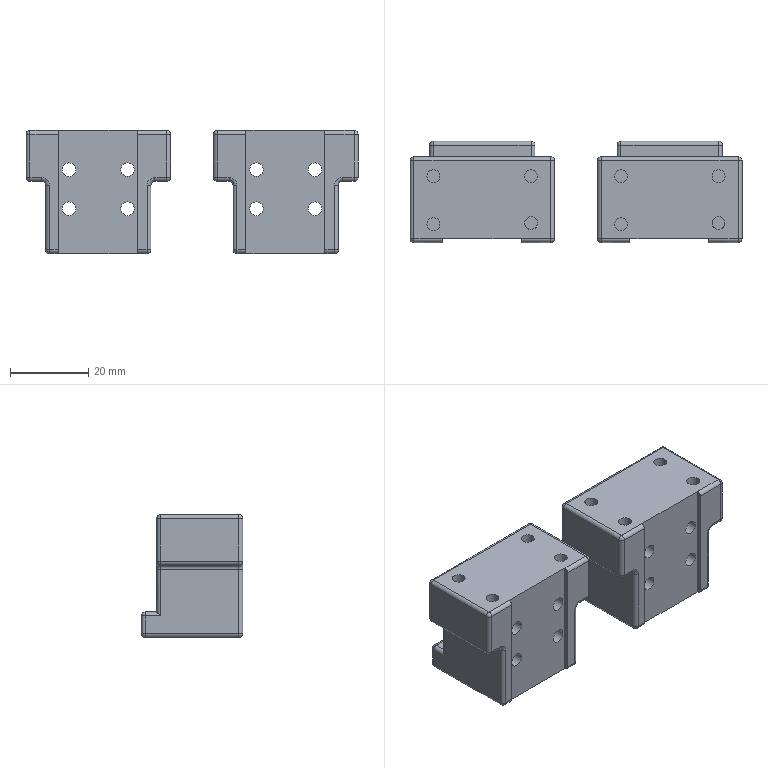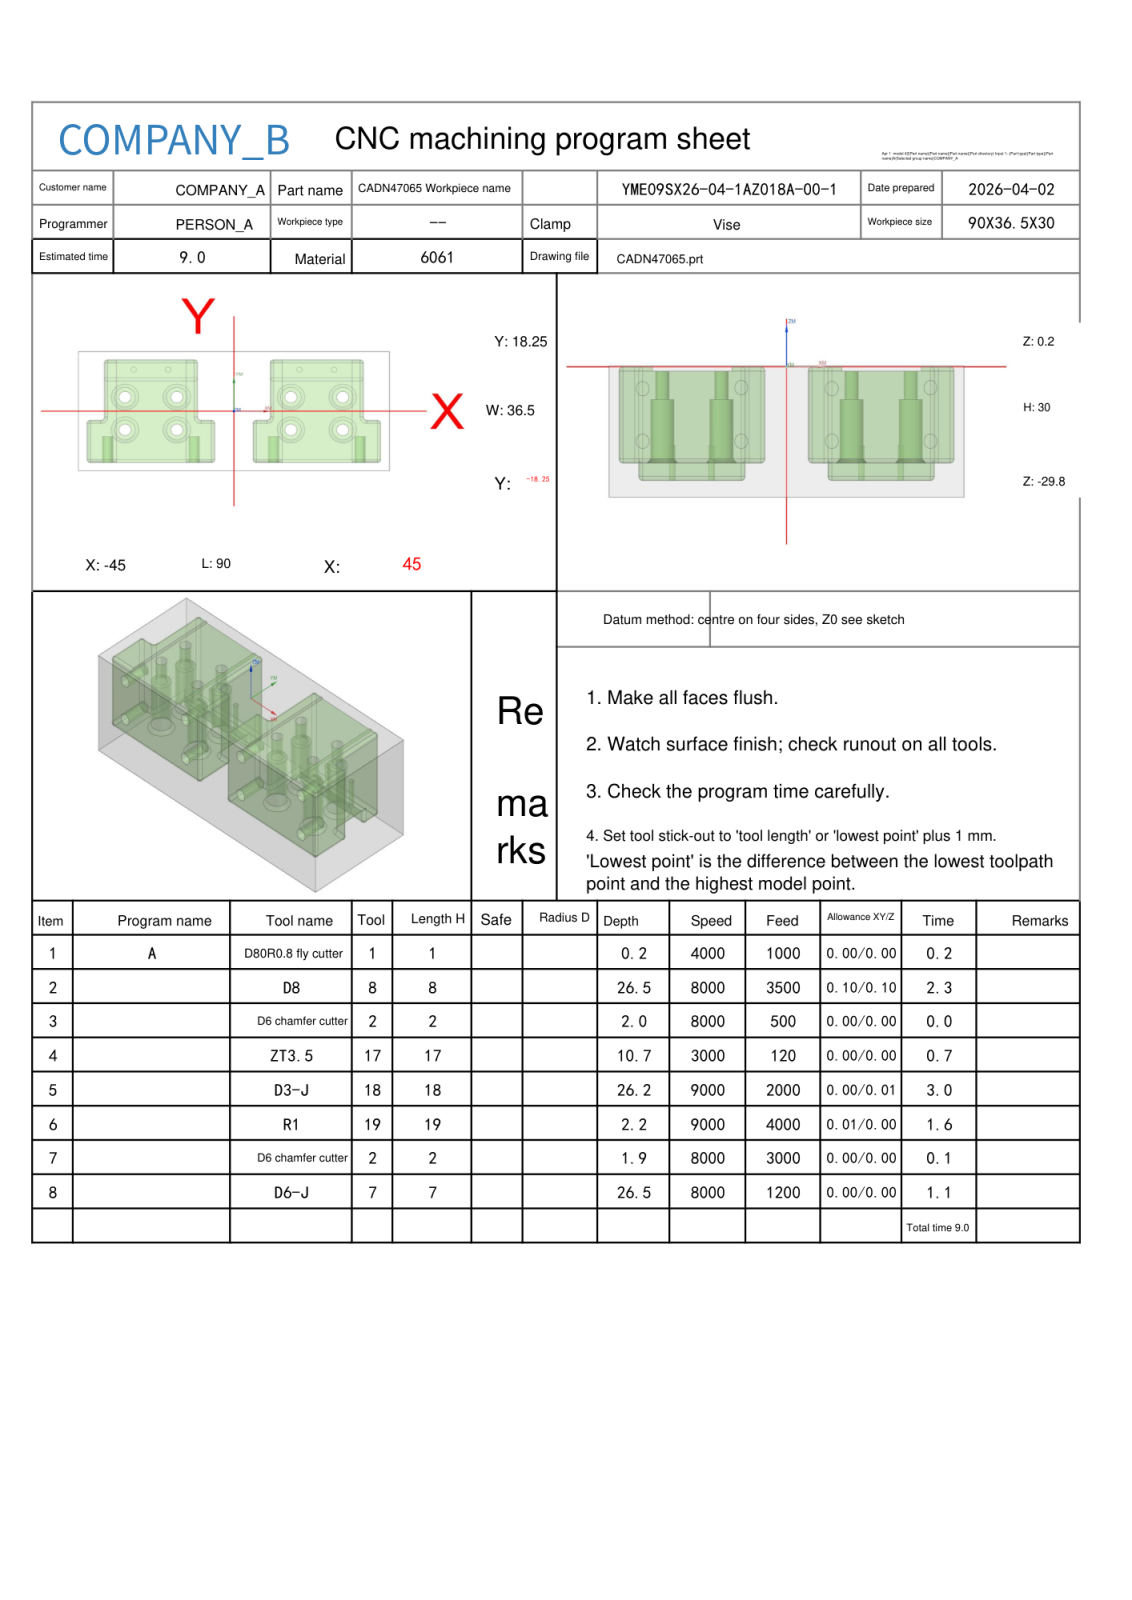NC program | NX | posted by the shop | part box 85 x 26 x 31.5 mm
Lines 3034 to 3073 of 17928:
N3 T02 M06
(D6 chamfer cutter  D=6. R=0. H=02 ce=0.00 di=0.10)
G00 G90 G54 X31.498 Y4.3 M03 S8000
G43 H02 Z20.
M08
G98 G81 X31.498 Y4.3 Z-1.8 R0.0 F500.
Y-5.7
X16.498
Y4.3
X-16.502
Y-5.7
X-31.502
Y4.3
G80
G00 Z20.
G91 G28 Z0.0
M05
M09
G91 G28 Z0.0
M01
N4 T17 M06
(ZT3.5 D=3.5 DR_a=118 H=17)
G00 G90 G54 X31.498 Y4.3 M03 S3000
G43 H17 Z20.
M08
G98 G83 X31.498 Y4.3 Z-10.542 R0.0 F120. Q3.
Y-5.7
X16.498
Y4.3
X-16.502
Y-5.7
X-31.502
Y4.3
G80
G00 Z20.
G91 G28 Z0.0
M05
M09
G91 G28 Z0.0
M01